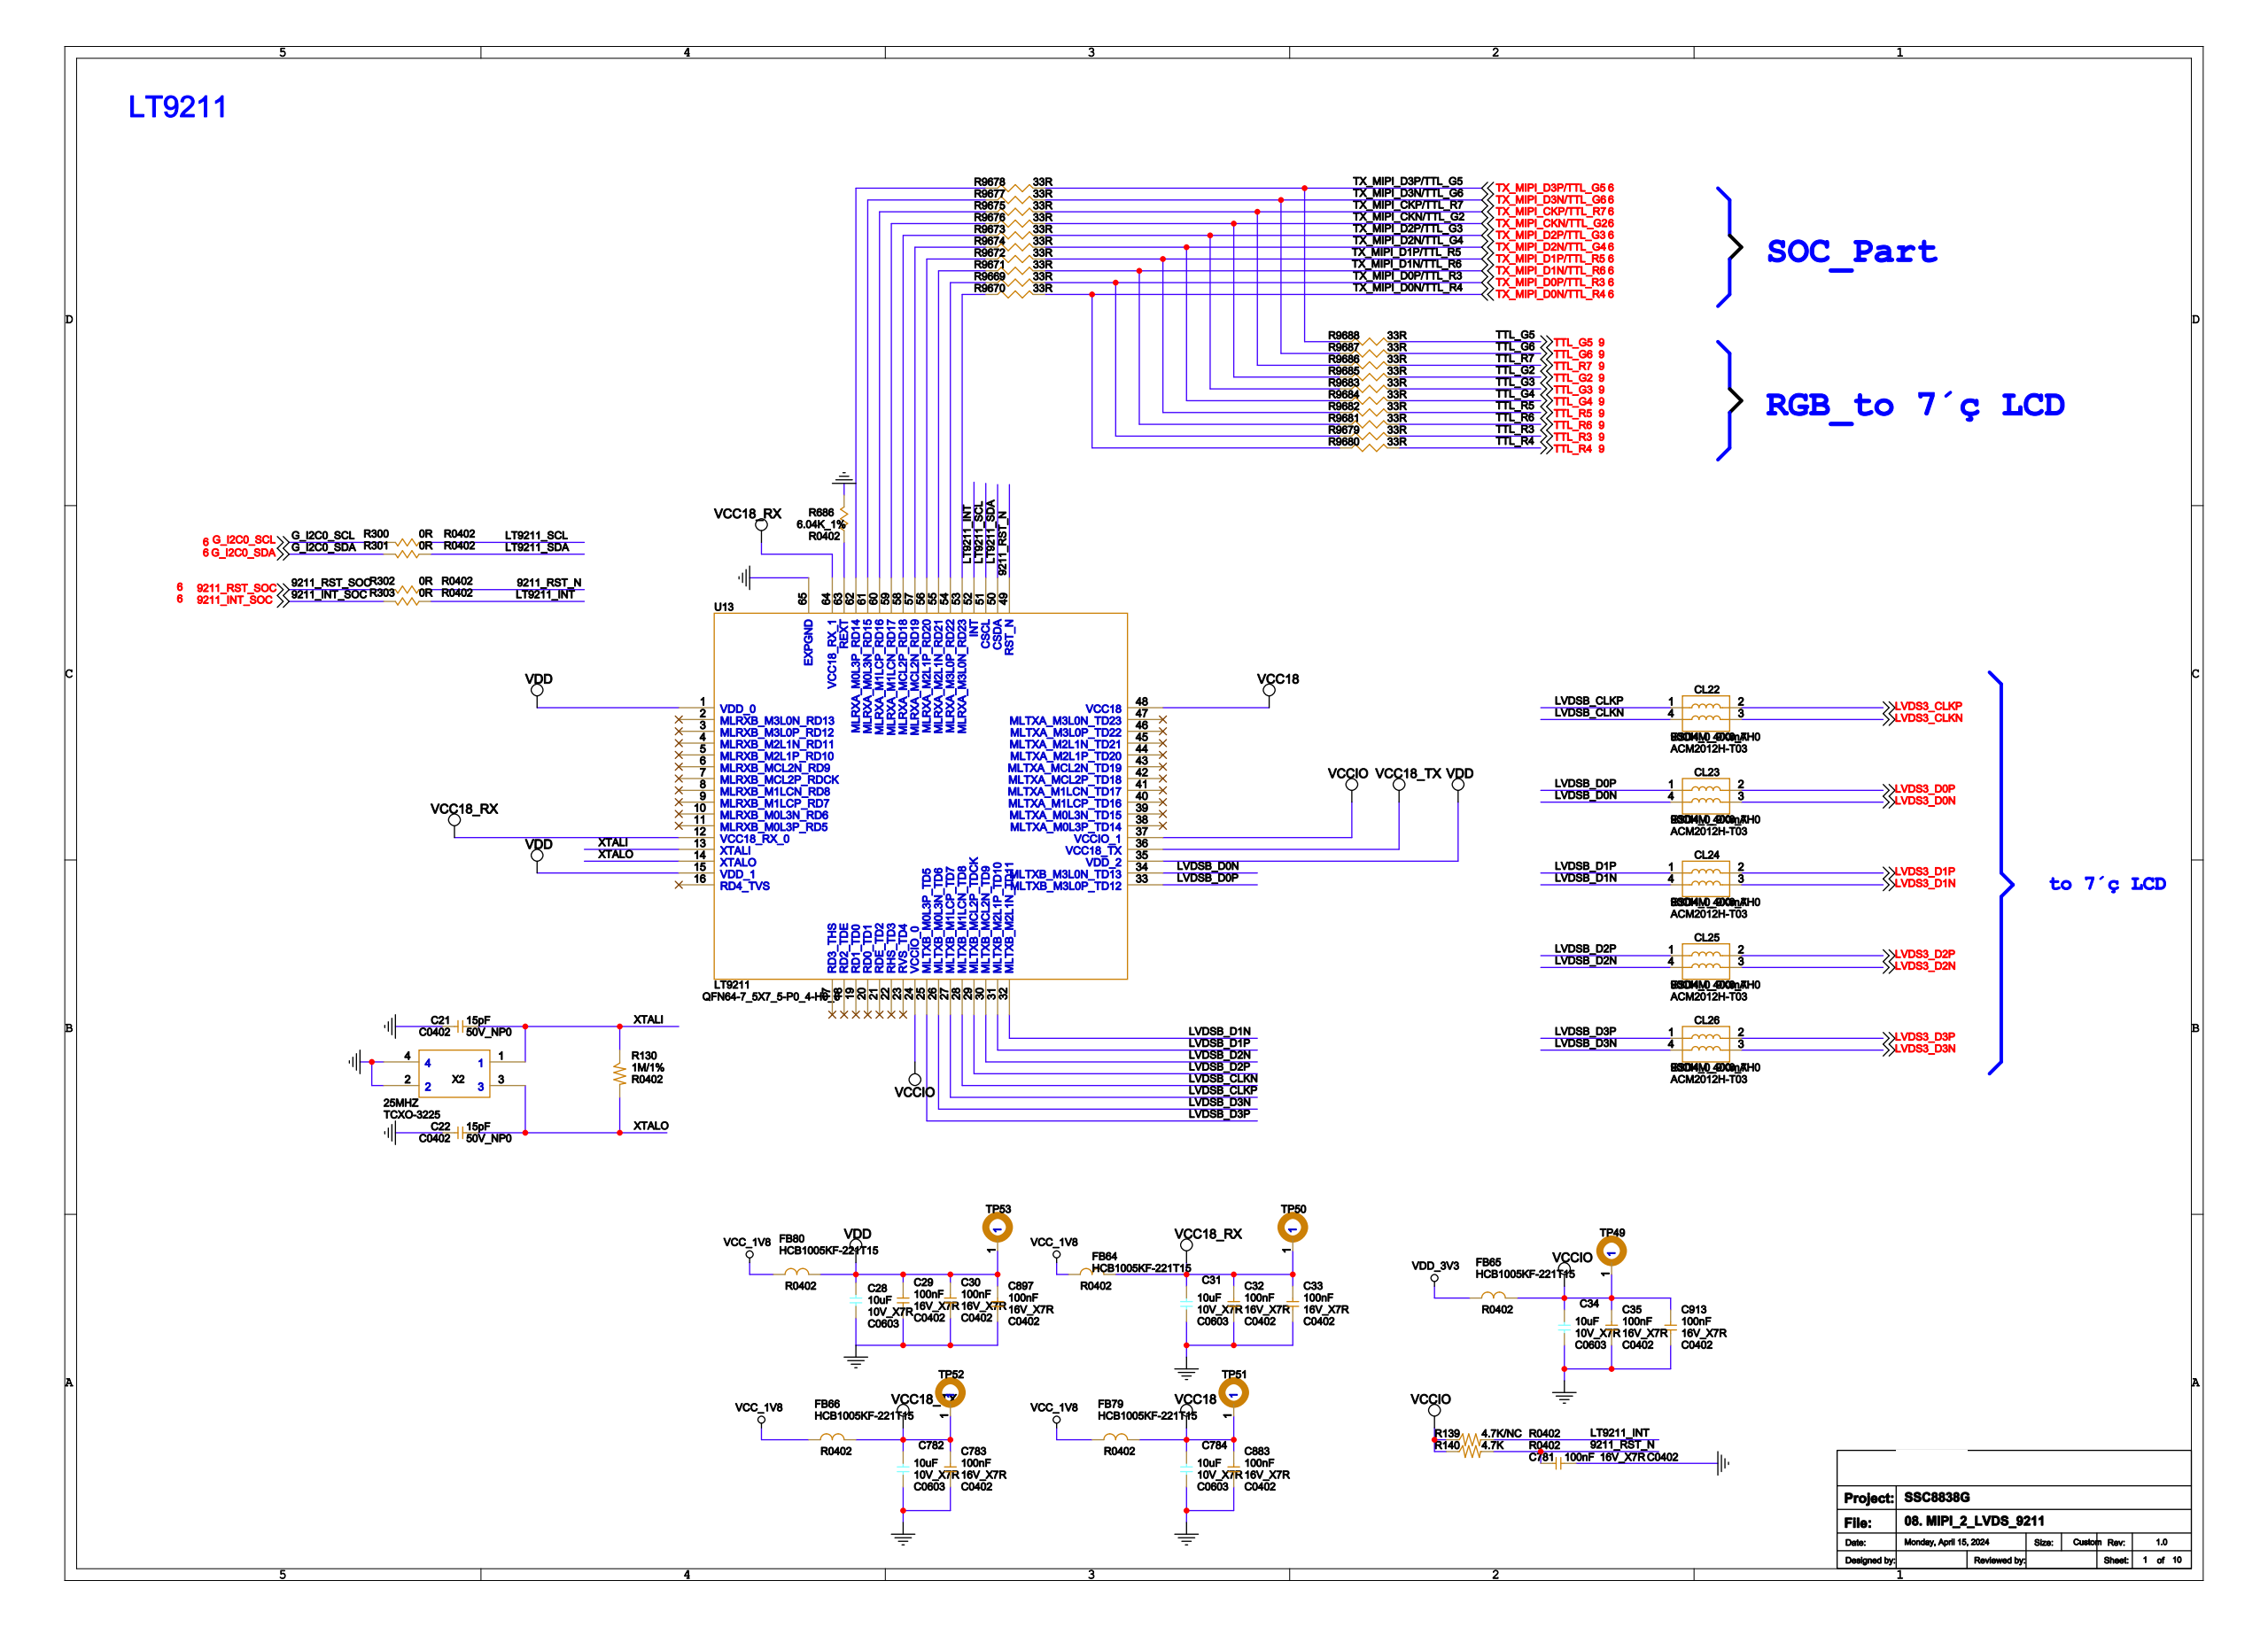Circuit board | Cadence Allegro | 958 parts | 601 nets | one sheet of the schematic
Parts on this sheet (reference | value | footprint):
C21 | 15pF | C0402
C22 | 15pF | C0402
C28 | 10uF | C0603
C29 | 100nF | C0402
C30 | 100nF | C0402
C31 | 10uF | C0603
C32 | 100nF | C0402
C33 | 100nF | C0402
C34 | 10uF | C0603
C35 | 100nF | C0402
C781 | 100nF | C0402
C782 | 10uF | C0603
C783 | 100nF | C0402
C784 | 10uF | C0603
C883 | 100nF | C0402
C897 | 100nF | C0402
C913 | 100nF | C0402
CL22 | 90OHM_400mA | ESD4_0_9X0_7H0
CL23 | 90OHM_400mA | ESD4_0_9X0_7H0
CL24 | 90OHM_400mA | ESD4_0_9X0_7H0
CL25 | 90OHM_400mA | ESD4_0_9X0_7H0
CL26 | 90OHM_400mA | ESD4_0_9X0_7H0
FB64 | HCB1005KF-221T15 | R0402
FB65 | HCB1005KF-221T15 | R0402
FB66 | HCB1005KF-221T15 | R0402
FB79 | HCB1005KF-221T15 | R0402
FB80 | HCB1005KF-221T15 | R0402
R130 | 1M/1% | R0402
R139 | 4.7K/NC | R0402
R140 | 4.7K | R0402
R300 | 0R | R0402
R301 | 0R | R0402
R302 | 0R | R0402
R303 | 0R | R0402
R686 | 6.04K_1% | R0402
R9669 | 33R | R0402
R9670 | 33R | R0402
R9671 | 33R | R0402
R9672 | 33R | R0402
R9673 | 33R | R0402
R9674 | 33R | R0402
R9675 | 33R | R0402
R9676 | 33R | R0402
R9677 | 33R | R0402
R9678 | 33R | R0402
R9679 | 33R | R0402
R9680 | 33R | R0402
R9681 | 33R | R0402
R9682 | 33R | R0402
R9683 | 33R | R0402
R9684 | 33R | R0402
R9685 | 33R | R0402
R9686 | 33R | R0402
R9687 | 33R | R0402
R9688 | 33R | R0402
TP49 | HOLE | TP_0R50
TP50 | HOLE | TP_0R50
TP51 | HOLE | TP_0R50
TP52 | HOLE | TP_0R50
TP53 | HOLE | TP_0R50
U13 | LT9211 | QFN64-7_5X7_5-P0_4-H0_8
X2 | 25MHZ | TCXO-3225
Nets of these parts (net: part-pin ...):
GND: C21-1 C22-1 C28-1 C29-1 C30-1 C31-1 C32-1 C33-1 C34-1 C35-1 C781-1 C782-1 C783-1 C784-1 C883-1 C897-1 C913-1 R686-2 X2-2 X2-4 U13-65
3V3_NORMAL: FB65-1
VDD: C28-2 C29-2 C30-2 C897-2 FB80-2 TP53-1 U13-1 U13-15 U13-35
VCC18_RX: C31-2 C32-2 C33-2 FB64-2 TP50-1 U13-12 U13-64
VCCIO: C34-2 C35-2 C913-2 FB65-2 R139-2 R140-2 TP49-1 U13-24 U13-37
9211_RST_N: C781-2 R140-1 R302-1 U13-49
VCC18_TX: C782-2 C783-2 FB66-2 TP52-1 U13-36
VCC18: C784-2 C883-2 FB79-2 TP51-1 U13-48
XTALI_19540032: C21-2 R130-2 X2-1 U13-13
XTALO_19540037: C22-2 R130-1 X2-3 U13-14
LVDSB_CLKP: CL22-1 U13-27
LVDS3_CLKP: CL22-2
LVDS3_CLKN: CL22-3
LVDSB_CLKN: CL22-4 U13-28
LVDSB_D0P: CL23-1 U13-33
LVDS3_D0P: CL23-2
LVDS3_D0N: CL23-3
LVDSB_D0N: CL23-4 U13-34
LVDSB_D1P: CL24-1 U13-31
LVDS3_D1P: CL24-2
LVDS3_D1N: CL24-3
LVDSB_D1N: CL24-4 U13-32
LVDSB_D2P: CL25-1 U13-29
LVDS3_D2P: CL25-2
LVDS3_D2N: CL25-3
LVDSB_D2N: CL25-4 U13-30
LVDSB_D3P: CL26-1 U13-25
LVDS3_D3P: CL26-2
LVDS3_D3N: CL26-3
LVDSB_D3N: CL26-4 U13-26
TTL_G2: R9685-2
TTL_G3: R9683-2
TTL_G4: R9684-2
TTL_G5: R9688-2
TTL_G6: R9687-2
TTL_R3: R9679-2
TTL_R4: R9680-2
TTL_R5: R9682-2
TTL_R6: R9681-2
TTL_R7: R9686-2
1V8: FB64-1 FB66-1 FB79-1 FB80-1
LT9211_INT: R139-1 R303-1 U13-52
LT9211_SCL: R300-1 U13-51
G_I2C0_SCL: R300-2
LT9211_SDA: R301-1 U13-50
G_I2C0_SDA: R301-2
9211_RST_SOC: R302-2
9211_INT_SOC: R303-2
N19539761: R686-1 U13-63
N21304753: R9669-1 U13-54
TX_MIPI_D0P/TTL_R3: R9669-2 R9679-1
N21304759: R9670-1 U13-53
TX_MIPI_D0N/TTL_R4: R9670-2 R9680-1
N21305836: R9671-1 U13-55
TX_MIPI_D1N/TTL_R6: R9671-2 R9681-1
N21305833: R9672-1 U13-56
TX_MIPI_D1P/TTL_R5: R9672-2 R9682-1
N21305797: R9673-1 U13-58
TX_MIPI_D2P/TTL_G3: R9673-2 R9683-1
N21305800: R9674-1 U13-57
TX_MIPI_D2N/TTL_G4: R9674-2 R9684-1
N21305761: R9675-1 U13-60
TX_MIPI_CKP/TTL_R7: R9675-2 R9686-1
N21305764: R9676-1 U13-59
TX_MIPI_CKN/TTL_G2: R9676-2 R9685-1
N21304777: R9677-1 U13-61
TX_MIPI_D3N/TTL_G6: R9677-2 R9687-1
N21304780: R9678-1 U13-62
TX_MIPI_D3P/TTL_G5: R9678-2 R9688-1